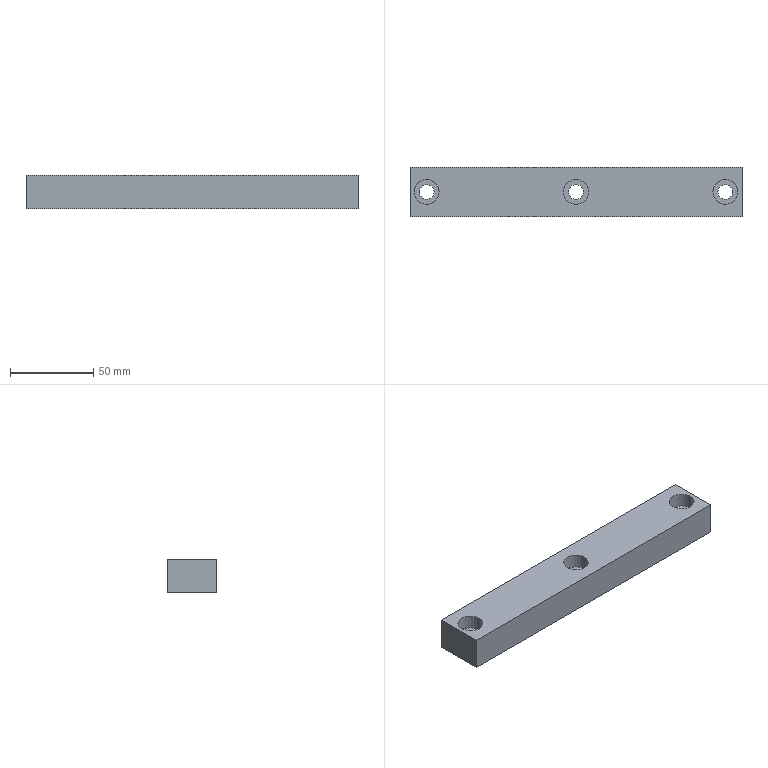Part | SolidWorks | features Extrusion 1, HoleWzd 1 | 1 solid | 21 faces | box 200 x 30 x 20 mm | volume 113265 mm3 | cylinder 12 | plane 9 | commonest cylinder face diameters 9 x6 15 x6
STEP:
#1=CARTESIAN_POINT('',(-7.5,0.,11.4));
#2=VERTEX_POINT('',#1);
#3=CARTESIAN_POINT('',(7.5,0.,11.4));
#4=VERTEX_POINT('',#3);
#5=CARTESIAN_POINT('',(0.,0.,11.4));
#6=DIRECTION('',(0.,0.,1.));
#7=DIRECTION('',(1.,0.,0.));
#8=AXIS2_PLACEMENT_3D('',#5,#6,#7);
#9=CIRCLE('',#8,7.5);
#10=EDGE_CURVE('',#2,#4,#9,.T.);
#11=ORIENTED_EDGE('',*,*,#10,.F.);
#12=CARTESIAN_POINT('',(-7.5,0.,20.));
#13=VERTEX_POINT('',#12);
#14=CARTESIAN_POINT('',(-7.5,0.,20.));
#15=DIRECTION('',(0.,0.,1.));
#16=VECTOR('',#15,1000.);
#17=LINE('',#14,#16);
#18=EDGE_CURVE('',#2,#13,#17,.T.);
#19=ORIENTED_EDGE('',*,*,#18,.T.);
#20=CARTESIAN_POINT('',(7.5,0.,20.));
#21=VERTEX_POINT('',#20);
#22=CARTESIAN_POINT('',(0.,0.,20.));
#23=DIRECTION('',(0.,0.,1.));
#24=DIRECTION('',(1.,0.,0.));
#25=AXIS2_PLACEMENT_3D('',#22,#23,#24);
#26=CIRCLE('',#25,7.5);
#27=EDGE_CURVE('',#13,#21,#26,.T.);
#28=ORIENTED_EDGE('',*,*,#27,.T.);
#29=CARTESIAN_POINT('',(7.5,0.,20.));
#30=DIRECTION('',(0.,0.,1.));
#31=VECTOR('',#30,1000.);
#32=LINE('',#29,#31);
#33=EDGE_CURVE('',#4,#21,#32,.T.);
#34=ORIENTED_EDGE('',*,*,#33,.F.);
#35=EDGE_LOOP('',(#11,#19,#28,#34));
#36=FACE_OUTER_BOUND('',#35,.T.);
#37=CARTESIAN_POINT('',(0.,0.,20.));
#38=DIRECTION('',(0.,0.,1.));
#39=DIRECTION('',(1.,0.,0.));
#40=AXIS2_PLACEMENT_3D('',#37,#38,#39);
#41=CYLINDRICAL_SURFACE('',#40,7.5);
#42=ADVANCED_FACE('',(#36),#41,.F.);
#43=CARTESIAN_POINT('',(-4.5,0.,0.));
#44=VERTEX_POINT('',#43);
#45=CARTESIAN_POINT('',(4.5,0.,0.));
#46=VERTEX_POINT('',#45);
#47=CARTESIAN_POINT('',(0.,0.,0.));
#48=DIRECTION('',(0.,0.,1.));
#49=DIRECTION('',(1.,0.,0.));
#50=AXIS2_PLACEMENT_3D('',#47,#48,#49);
#51=CIRCLE('',#50,4.5);
#52=EDGE_CURVE('',#44,#46,#51,.T.);
#53=ORIENTED_EDGE('',*,*,#52,.F.);
#54=CARTESIAN_POINT('',(-4.5,0.,11.4));
#55=VERTEX_POINT('',#54);
#56=CARTESIAN_POINT('',(-4.5,0.,20.));
#57=DIRECTION('',(0.,0.,1.));
#58=VECTOR('',#57,1000.);
#59=LINE('',#56,#58);
#60=EDGE_CURVE('',#44,#55,#59,.T.);
#61=ORIENTED_EDGE('',*,*,#60,.T.);
#62=CARTESIAN_POINT('',(4.5,0.,11.4));
#63=VERTEX_POINT('',#62);
#64=CARTESIAN_POINT('',(0.,0.,11.4));
#65=DIRECTION('',(0.,0.,1.));
#66=DIRECTION('',(1.,0.,0.));
#67=AXIS2_PLACEMENT_3D('',#64,#65,#66);
#68=CIRCLE('',#67,4.5);
#69=EDGE_CURVE('',#55,#63,#68,.T.);
#70=ORIENTED_EDGE('',*,*,#69,.T.);
#71=CARTESIAN_POINT('',(4.5,0.,20.));
#72=DIRECTION('',(0.,0.,1.));
#73=VECTOR('',#72,1000.);
#74=LINE('',#71,#73);
#75=EDGE_CURVE('',#46,#63,#74,.T.);
#76=ORIENTED_EDGE('',*,*,#75,.F.);
#77=EDGE_LOOP('',(#53,#61,#70,#76));
#78=FACE_OUTER_BOUND('',#77,.T.);
#79=CARTESIAN_POINT('',(0.,0.,20.));
#80=DIRECTION('',(0.,0.,1.));
#81=DIRECTION('',(1.,0.,0.));
#82=AXIS2_PLACEMENT_3D('',#79,#80,#81);
#83=CYLINDRICAL_SURFACE('',#82,4.5);
#84=ADVANCED_FACE('',(#78),#83,.F.);
#85=CARTESIAN_POINT('',(82.5,0.,11.4));
#86=VERTEX_POINT('',#85);
#87=CARTESIAN_POINT('',(97.5,0.,11.4));
#88=VERTEX_POINT('',#87);
#89=CARTESIAN_POINT('',(90.,0.,11.4));
#90=DIRECTION('',(0.,0.,1.));
#91=DIRECTION('',(1.,0.,0.));
#92=AXIS2_PLACEMENT_3D('',#89,#90,#91);
#93=CIRCLE('',#92,7.5);
#94=EDGE_CURVE('',#86,#88,#93,.T.);
#95=ORIENTED_EDGE('',*,*,#94,.F.);
#96=CARTESIAN_POINT('',(82.5,0.,20.));
#97=VERTEX_POINT('',#96);
#98=CARTESIAN_POINT('',(82.5,0.,20.));
#99=DIRECTION('',(0.,0.,1.));
#100=VECTOR('',#99,1000.);
#101=LINE('',#98,#100);
#102=EDGE_CURVE('',#86,#97,#101,.T.);
#103=ORIENTED_EDGE('',*,*,#102,.T.);
#104=CARTESIAN_POINT('',(97.5,0.,20.));
#105=VERTEX_POINT('',#104);
#106=CARTESIAN_POINT('',(90.,0.,20.));
#107=DIRECTION('',(0.,0.,1.));
#108=DIRECTION('',(1.,0.,0.));
#109=AXIS2_PLACEMENT_3D('',#106,#107,#108);
#110=CIRCLE('',#109,7.5);
#111=EDGE_CURVE('',#97,#105,#110,.T.);
#112=ORIENTED_EDGE('',*,*,#111,.T.);
#113=CARTESIAN_POINT('',(97.5,0.,20.));
#114=DIRECTION('',(0.,0.,1.));
#115=VECTOR('',#114,1000.);
#116=LINE('',#113,#115);
#117=EDGE_CURVE('',#88,#105,#116,.T.);
#118=ORIENTED_EDGE('',*,*,#117,.F.);
#119=EDGE_LOOP('',(#95,#103,#112,#118));
#120=FACE_OUTER_BOUND('',#119,.T.);
#121=CARTESIAN_POINT('',(90.,0.,20.));
#122=DIRECTION('',(0.,0.,1.));
#123=DIRECTION('',(1.,0.,0.));
#124=AXIS2_PLACEMENT_3D('',#121,#122,#123);
#125=CYLINDRICAL_SURFACE('',#124,7.5);
#126=ADVANCED_FACE('',(#120),#125,.F.);
#127=CARTESIAN_POINT('',(85.5,0.,0.));
#128=VERTEX_POINT('',#127);
#129=CARTESIAN_POINT('',(94.5,0.,0.));
#130=VERTEX_POINT('',#129);
#131=CARTESIAN_POINT('',(90.,0.,0.));
#132=DIRECTION('',(0.,0.,1.));
#133=DIRECTION('',(1.,0.,0.));
#134=AXIS2_PLACEMENT_3D('',#131,#132,#133);
#135=CIRCLE('',#134,4.5);
#136=EDGE_CURVE('',#128,#130,#135,.T.);
#137=ORIENTED_EDGE('',*,*,#136,.F.);
#138=CARTESIAN_POINT('',(85.5,0.,11.4));
#139=VERTEX_POINT('',#138);
#140=CARTESIAN_POINT('',(85.5,0.,20.));
#141=DIRECTION('',(0.,0.,1.));
#142=VECTOR('',#141,1000.);
#143=LINE('',#140,#142);
#144=EDGE_CURVE('',#128,#139,#143,.T.);
#145=ORIENTED_EDGE('',*,*,#144,.T.);
#146=CARTESIAN_POINT('',(94.5,0.,11.4));
#147=VERTEX_POINT('',#146);
#148=CARTESIAN_POINT('',(90.,0.,11.4));
#149=DIRECTION('',(0.,0.,1.));
#150=DIRECTION('',(1.,0.,0.));
#151=AXIS2_PLACEMENT_3D('',#148,#149,#150);
#152=CIRCLE('',#151,4.5);
#153=EDGE_CURVE('',#139,#147,#152,.T.);
#154=ORIENTED_EDGE('',*,*,#153,.T.);
#155=CARTESIAN_POINT('',(94.5,0.,20.));
#156=DIRECTION('',(0.,0.,1.));
#157=VECTOR('',#156,1000.);
#158=LINE('',#155,#157);
#159=EDGE_CURVE('',#130,#147,#158,.T.);
#160=ORIENTED_EDGE('',*,*,#159,.F.);
#161=EDGE_LOOP('',(#137,#145,#154,#160));
#162=FACE_OUTER_BOUND('',#161,.T.);
#163=CARTESIAN_POINT('',(90.,0.,20.));
#164=DIRECTION('',(0.,0.,1.));
#165=DIRECTION('',(1.,0.,0.));
#166=AXIS2_PLACEMENT_3D('',#163,#164,#165);
#167=CYLINDRICAL_SURFACE('',#166,4.5);
#168=ADVANCED_FACE('',(#162),#167,.F.);
#169=CARTESIAN_POINT('',(-97.5,0.,11.4));
#170=VERTEX_POINT('',#169);
#171=CARTESIAN_POINT('',(-82.5,0.,11.4));
#172=VERTEX_POINT('',#171);
#173=CARTESIAN_POINT('',(-90.,0.,11.4));
#174=DIRECTION('',(0.,0.,1.));
#175=DIRECTION('',(1.,0.,0.));
#176=AXIS2_PLACEMENT_3D('',#173,#174,#175);
#177=CIRCLE('',#176,7.5);
#178=EDGE_CURVE('',#170,#172,#177,.T.);
#179=ORIENTED_EDGE('',*,*,#178,.F.);
#180=CARTESIAN_POINT('',(-97.5,0.,20.));
#181=VERTEX_POINT('',#180);
#182=CARTESIAN_POINT('',(-97.5,0.,20.));
#183=DIRECTION('',(0.,0.,1.));
#184=VECTOR('',#183,1000.);
#185=LINE('',#182,#184);
#186=EDGE_CURVE('',#170,#181,#185,.T.);
#187=ORIENTED_EDGE('',*,*,#186,.T.);
#188=CARTESIAN_POINT('',(-82.5,0.,20.));
#189=VERTEX_POINT('',#188);
#190=CARTESIAN_POINT('',(-90.,0.,20.));
#191=DIRECTION('',(0.,0.,1.));
#192=DIRECTION('',(1.,0.,0.));
#193=AXIS2_PLACEMENT_3D('',#190,#191,#192);
#194=CIRCLE('',#193,7.5);
#195=EDGE_CURVE('',#181,#189,#194,.T.);
#196=ORIENTED_EDGE('',*,*,#195,.T.);
#197=CARTESIAN_POINT('',(-82.5,0.,20.));
#198=DIRECTION('',(0.,0.,1.));
#199=VECTOR('',#198,1000.);
#200=LINE('',#197,#199);
#201=EDGE_CURVE('',#172,#189,#200,.T.);
#202=ORIENTED_EDGE('',*,*,#201,.F.);
#203=EDGE_LOOP('',(#179,#187,#196,#202));
#204=FACE_OUTER_BOUND('',#203,.T.);
#205=CARTESIAN_POINT('',(-90.,0.,20.));
#206=DIRECTION('',(0.,0.,1.));
#207=DIRECTION('',(1.,0.,0.));
#208=AXIS2_PLACEMENT_3D('',#205,#206,#207);
#209=CYLINDRICAL_SURFACE('',#208,7.5);
#210=ADVANCED_FACE('',(#204),#209,.F.);
#211=CARTESIAN_POINT('',(-94.5,0.,0.));
#212=VERTEX_POINT('',#211);
#213=CARTESIAN_POINT('',(-85.5,0.,0.));
#214=VERTEX_POINT('',#213);
#215=CARTESIAN_POINT('',(-90.,0.,0.));
#216=DIRECTION('',(0.,0.,1.));
#217=DIRECTION('',(1.,0.,0.));
#218=AXIS2_PLACEMENT_3D('',#215,#216,#217);
#219=CIRCLE('',#218,4.5);
#220=EDGE_CURVE('',#212,#214,#219,.T.);
#221=ORIENTED_EDGE('',*,*,#220,.F.);
#222=CARTESIAN_POINT('',(-94.5,0.,11.4));
#223=VERTEX_POINT('',#222);
#224=CARTESIAN_POINT('',(-94.5,0.,20.));
#225=DIRECTION('',(0.,0.,1.));
#226=VECTOR('',#225,1000.);
#227=LINE('',#224,#226);
#228=EDGE_CURVE('',#212,#223,#227,.T.);
#229=ORIENTED_EDGE('',*,*,#228,.T.);
#230=CARTESIAN_POINT('',(-85.5,0.,11.4));
#231=VERTEX_POINT('',#230);
#232=CARTESIAN_POINT('',(-90.,0.,11.4));
#233=DIRECTION('',(0.,0.,1.));
#234=DIRECTION('',(1.,0.,0.));
#235=AXIS2_PLACEMENT_3D('',#232,#233,#234);
#236=CIRCLE('',#235,4.5);
#237=EDGE_CURVE('',#223,#231,#236,.T.);
#238=ORIENTED_EDGE('',*,*,#237,.T.);
#239=CARTESIAN_POINT('',(-85.5,0.,20.));
#240=DIRECTION('',(0.,0.,1.));
#241=VECTOR('',#240,1000.);
#242=LINE('',#239,#241);
#243=EDGE_CURVE('',#214,#231,#242,.T.);
#244=ORIENTED_EDGE('',*,*,#243,.F.);
#245=EDGE_LOOP('',(#221,#229,#238,#244));
#246=FACE_OUTER_BOUND('',#245,.T.);
#247=CARTESIAN_POINT('',(-90.,0.,20.));
#248=DIRECTION('',(0.,0.,1.));
#249=DIRECTION('',(1.,0.,0.));
#250=AXIS2_PLACEMENT_3D('',#247,#248,#249);
#251=CYLINDRICAL_SURFACE('',#250,4.5);
#252=ADVANCED_FACE('',(#246),#251,.F.);
#253=CARTESIAN_POINT('',(100.,-15.,0.));
#254=VERTEX_POINT('',#253);
#255=CARTESIAN_POINT('',(100.,15.,0.));
#256=VERTEX_POINT('',#255);
#257=CARTESIAN_POINT('',(100.,-15.,0.));
#258=DIRECTION('',(0.,1.,0.));
#259=VECTOR('',#258,1000.);
#260=LINE('',#257,#259);
#261=EDGE_CURVE('',#254,#256,#260,.T.);
#262=ORIENTED_EDGE('',*,*,#261,.T.);
#263=CARTESIAN_POINT('',(100.,15.,20.));
#264=VERTEX_POINT('',#263);
#265=CARTESIAN_POINT('',(100.,15.,20.));
#266=DIRECTION('',(0.,0.,-1.));
#267=VECTOR('',#266,1000.);
#268=LINE('',#265,#267);
#269=EDGE_CURVE('',#264,#256,#268,.T.);
#270=ORIENTED_EDGE('',*,*,#269,.F.);
#271=CARTESIAN_POINT('',(100.,-15.,20.));
#272=VERTEX_POINT('',#271);
#273=CARTESIAN_POINT('',(100.,-15.,20.));
#274=DIRECTION('',(0.,1.,0.));
#275=VECTOR('',#274,1000.);
#276=LINE('',#273,#275);
#277=EDGE_CURVE('',#272,#264,#276,.T.);
#278=ORIENTED_EDGE('',*,*,#277,.F.);
#279=CARTESIAN_POINT('',(100.,-15.,20.));
#280=DIRECTION('',(0.,0.,-1.));
#281=VECTOR('',#280,1000.);
#282=LINE('',#279,#281);
#283=EDGE_CURVE('',#272,#254,#282,.T.);
#284=ORIENTED_EDGE('',*,*,#283,.T.);
#285=EDGE_LOOP('',(#262,#270,#278,#284));
#286=FACE_OUTER_BOUND('',#285,.T.);
#287=CARTESIAN_POINT('',(100.,-15.,20.));
#288=DIRECTION('',(-1.,0.,0.));
#289=DIRECTION('',(0.,0.,1.));
#290=AXIS2_PLACEMENT_3D('',#287,#288,#289);
#291=PLANE('',#290);
#292=ADVANCED_FACE('',(#286),#291,.F.);
#293=CARTESIAN_POINT('',(-100.,15.,0.));
#294=VERTEX_POINT('',#293);
#295=CARTESIAN_POINT('',(-100.,15.,0.));
#296=DIRECTION('',(-1.,0.,0.));
#297=VECTOR('',#296,1000.);
#298=LINE('',#295,#297);
#299=EDGE_CURVE('',#256,#294,#298,.T.);
#300=ORIENTED_EDGE('',*,*,#299,.T.);
#301=CARTESIAN_POINT('',(-100.,15.,20.));
#302=VERTEX_POINT('',#301);
#303=CARTESIAN_POINT('',(-100.,15.,20.));
#304=DIRECTION('',(0.,0.,-1.));
#305=VECTOR('',#304,1000.);
#306=LINE('',#303,#305);
#307=EDGE_CURVE('',#302,#294,#306,.T.);
#308=ORIENTED_EDGE('',*,*,#307,.F.);
#309=CARTESIAN_POINT('',(-100.,15.,20.));
#310=DIRECTION('',(-1.,0.,0.));
#311=VECTOR('',#310,1000.);
#312=LINE('',#309,#311);
#313=EDGE_CURVE('',#264,#302,#312,.T.);
#314=ORIENTED_EDGE('',*,*,#313,.F.);
#315=ORIENTED_EDGE('',*,*,#269,.T.);
#316=EDGE_LOOP('',(#300,#308,#314,#315));
#317=FACE_OUTER_BOUND('',#316,.T.);
#318=CARTESIAN_POINT('',(-100.,15.,20.));
#319=DIRECTION('',(0.,-1.,0.));
#320=DIRECTION('',(0.,0.,-1.));
#321=AXIS2_PLACEMENT_3D('',#318,#319,#320);
#322=PLANE('',#321);
#323=ADVANCED_FACE('',(#317),#322,.F.);
#324=CARTESIAN_POINT('',(-100.,-15.,0.));
#325=VERTEX_POINT('',#324);
#326=CARTESIAN_POINT('',(-100.,-15.,0.));
#327=DIRECTION('',(0.,-1.,0.));
#328=VECTOR('',#327,1000.);
#329=LINE('',#326,#328);
#330=EDGE_CURVE('',#294,#325,#329,.T.);
#331=ORIENTED_EDGE('',*,*,#330,.T.);
#332=CARTESIAN_POINT('',(-100.,-15.,20.));
#333=VERTEX_POINT('',#332);
#334=CARTESIAN_POINT('',(-100.,-15.,20.));
#335=DIRECTION('',(0.,0.,-1.));
#336=VECTOR('',#335,1000.);
#337=LINE('',#334,#336);
#338=EDGE_CURVE('',#333,#325,#337,.T.);
#339=ORIENTED_EDGE('',*,*,#338,.F.);
#340=CARTESIAN_POINT('',(-100.,-15.,20.));
#341=DIRECTION('',(0.,-1.,0.));
#342=VECTOR('',#341,1000.);
#343=LINE('',#340,#342);
#344=EDGE_CURVE('',#302,#333,#343,.T.);
#345=ORIENTED_EDGE('',*,*,#344,.F.);
#346=ORIENTED_EDGE('',*,*,#307,.T.);
#347=EDGE_LOOP('',(#331,#339,#345,#346));
#348=FACE_OUTER_BOUND('',#347,.T.);
#349=CARTESIAN_POINT('',(-100.,-15.,20.));
#350=DIRECTION('',(1.,0.,0.));
#351=DIRECTION('',(0.,0.,-1.));
#352=AXIS2_PLACEMENT_3D('',#349,#350,#351);
#353=PLANE('',#352);
#354=ADVANCED_FACE('',(#348),#353,.F.);
#355=CARTESIAN_POINT('',(-100.,-15.,0.));
#356=DIRECTION('',(1.,0.,0.));
#357=VECTOR('',#356,1000.);
#358=LINE('',#355,#357);
#359=EDGE_CURVE('',#325,#254,#358,.T.);
#360=ORIENTED_EDGE('',*,*,#359,.T.);
#361=ORIENTED_EDGE('',*,*,#283,.F.);
#362=CARTESIAN_POINT('',(-100.,-15.,20.));
#363=DIRECTION('',(1.,0.,0.));
#364=VECTOR('',#363,1000.);
#365=LINE('',#362,#364);
#366=EDGE_CURVE('',#333,#272,#365,.T.);
#367=ORIENTED_EDGE('',*,*,#366,.F.);
#368=ORIENTED_EDGE('',*,*,#338,.T.);
#369=EDGE_LOOP('',(#360,#361,#367,#368));
#370=FACE_OUTER_BOUND('',#369,.T.);
#371=CARTESIAN_POINT('',(-100.,-15.,20.));
#372=DIRECTION('',(0.,1.,0.));
#373=DIRECTION('',(0.,0.,1.));
#374=AXIS2_PLACEMENT_3D('',#371,#372,#373);
#375=PLANE('',#374);
#376=ADVANCED_FACE('',(#370),#375,.F.);
#377=CARTESIAN_POINT('',(0.,0.,20.));
#378=DIRECTION('',(0.,0.,1.));
#379=DIRECTION('',(1.,0.,0.));
#380=AXIS2_PLACEMENT_3D('',#377,#378,#379);
#381=CIRCLE('',#380,7.5);
#382=EDGE_CURVE('',#21,#13,#381,.T.);
#383=ORIENTED_EDGE('',*,*,#382,.F.);
#384=ORIENTED_EDGE('',*,*,#27,.F.);
#385=EDGE_LOOP('',(#383,#384));
#386=FACE_BOUND('',#385,.T.);
#387=CARTESIAN_POINT('',(90.,0.,20.));
#388=DIRECTION('',(0.,0.,1.));
#389=DIRECTION('',(1.,0.,0.));
#390=AXIS2_PLACEMENT_3D('',#387,#388,#389);
#391=CIRCLE('',#390,7.5);
#392=EDGE_CURVE('',#105,#97,#391,.T.);
#393=ORIENTED_EDGE('',*,*,#392,.F.);
#394=ORIENTED_EDGE('',*,*,#111,.F.);
#395=EDGE_LOOP('',(#393,#394));
#396=FACE_BOUND('',#395,.T.);
#397=CARTESIAN_POINT('',(-90.,0.,20.));
#398=DIRECTION('',(0.,0.,1.));
#399=DIRECTION('',(1.,0.,0.));
#400=AXIS2_PLACEMENT_3D('',#397,#398,#399);
#401=CIRCLE('',#400,7.5);
#402=EDGE_CURVE('',#189,#181,#401,.T.);
#403=ORIENTED_EDGE('',*,*,#402,.F.);
#404=ORIENTED_EDGE('',*,*,#195,.F.);
#405=EDGE_LOOP('',(#403,#404));
#406=FACE_BOUND('',#405,.T.);
#407=ORIENTED_EDGE('',*,*,#277,.T.);
#408=ORIENTED_EDGE('',*,*,#313,.T.);
#409=ORIENTED_EDGE('',*,*,#344,.T.);
#410=ORIENTED_EDGE('',*,*,#366,.T.);
#411=EDGE_LOOP('',(#407,#408,#409,#410));
#412=FACE_OUTER_BOUND('',#411,.T.);
#413=CARTESIAN_POINT('',(0.,0.,20.));
#414=DIRECTION('',(0.,0.,-1.));
#415=DIRECTION('',(-1.,0.,0.));
#416=AXIS2_PLACEMENT_3D('',#413,#414,#415);
#417=PLANE('',#416);
#418=ADVANCED_FACE('',(#386,#396,#406,#412),#417,.F.);
#419=CARTESIAN_POINT('',(0.,0.,0.));
#420=DIRECTION('',(0.,0.,1.));
#421=DIRECTION('',(1.,0.,0.));
#422=AXIS2_PLACEMENT_3D('',#419,#420,#421);
#423=CIRCLE('',#422,4.5);
#424=EDGE_CURVE('',#46,#44,#423,.T.);
#425=ORIENTED_EDGE('',*,*,#424,.T.);
#426=ORIENTED_EDGE('',*,*,#52,.T.);
#427=EDGE_LOOP('',(#425,#426));
#428=FACE_BOUND('',#427,.T.);
#429=CARTESIAN_POINT('',(90.,0.,0.));
#430=DIRECTION('',(0.,0.,1.));
#431=DIRECTION('',(1.,0.,0.));
#432=AXIS2_PLACEMENT_3D('',#429,#430,#431);
#433=CIRCLE('',#432,4.5);
#434=EDGE_CURVE('',#130,#128,#433,.T.);
#435=ORIENTED_EDGE('',*,*,#434,.T.);
#436=ORIENTED_EDGE('',*,*,#136,.T.);
#437=EDGE_LOOP('',(#435,#436));
#438=FACE_BOUND('',#437,.T.);
#439=CARTESIAN_POINT('',(-90.,0.,0.));
#440=DIRECTION('',(0.,0.,1.));
#441=DIRECTION('',(1.,0.,0.));
#442=AXIS2_PLACEMENT_3D('',#439,#440,#441);
#443=CIRCLE('',#442,4.5);
#444=EDGE_CURVE('',#214,#212,#443,.T.);
#445=ORIENTED_EDGE('',*,*,#444,.T.);
#446=ORIENTED_EDGE('',*,*,#220,.T.);
#447=EDGE_LOOP('',(#445,#446));
#448=FACE_BOUND('',#447,.T.);
#449=ORIENTED_EDGE('',*,*,#261,.F.);
#450=ORIENTED_EDGE('',*,*,#359,.F.);
#451=ORIENTED_EDGE('',*,*,#330,.F.);
#452=ORIENTED_EDGE('',*,*,#299,.F.);
#453=EDGE_LOOP('',(#449,#450,#451,#452));
#454=FACE_OUTER_BOUND('',#453,.T.);
#455=CARTESIAN_POINT('',(0.,0.,0.));
#456=DIRECTION('',(0.,0.,-1.));
#457=DIRECTION('',(-1.,0.,0.));
#458=AXIS2_PLACEMENT_3D('',#455,#456,#457);
#459=PLANE('',#458);
#460=ADVANCED_FACE('',(#428,#438,#448,#454),#459,.T.);
#461=ORIENTED_EDGE('',*,*,#228,.F.);
#462=ORIENTED_EDGE('',*,*,#444,.F.);
#463=ORIENTED_EDGE('',*,*,#243,.T.);
#464=CARTESIAN_POINT('',(-90.,0.,11.4));
#465=DIRECTION('',(0.,0.,1.));
#466=DIRECTION('',(1.,0.,0.));
#467=AXIS2_PLACEMENT_3D('',#464,#465,#466);
#468=CIRCLE('',#467,4.5);
#469=EDGE_CURVE('',#231,#223,#468,.T.);
#470=ORIENTED_EDGE('',*,*,#469,.T.);
#471=EDGE_LOOP('',(#461,#462,#463,#470));
#472=FACE_OUTER_BOUND('',#471,.T.);
#473=CARTESIAN_POINT('',(-90.,0.,20.));
#474=DIRECTION('',(0.,0.,1.));
#475=DIRECTION('',(1.,0.,0.));
#476=AXIS2_PLACEMENT_3D('',#473,#474,#475);
#477=CYLINDRICAL_SURFACE('',#476,4.5);
#478=ADVANCED_FACE('',(#472),#477,.F.);
#479=ORIENTED_EDGE('',*,*,#469,.F.);
#480=ORIENTED_EDGE('',*,*,#237,.F.);
#481=EDGE_LOOP('',(#479,#480));
#482=FACE_BOUND('',#481,.T.);
#483=CARTESIAN_POINT('',(-90.,0.,11.4));
#484=DIRECTION('',(0.,0.,1.));
#485=DIRECTION('',(1.,0.,0.));
#486=AXIS2_PLACEMENT_3D('',#483,#484,#485);
#487=CIRCLE('',#486,7.5);
#488=EDGE_CURVE('',#172,#170,#487,.T.);
#489=ORIENTED_EDGE('',*,*,#488,.T.);
#490=ORIENTED_EDGE('',*,*,#178,.T.);
#491=EDGE_LOOP('',(#489,#490));
#492=FACE_OUTER_BOUND('',#491,.T.);
#493=CARTESIAN_POINT('',(-85.5,0.,11.4));
#494=DIRECTION('',(0.,0.,-1.));
#495=DIRECTION('',(-1.,0.,0.));
#496=AXIS2_PLACEMENT_3D('',#493,#494,#495);
#497=PLANE('',#496);
#498=ADVANCED_FACE('',(#482,#492),#497,.F.);
#499=ORIENTED_EDGE('',*,*,#186,.F.);
#500=ORIENTED_EDGE('',*,*,#488,.F.);
#501=ORIENTED_EDGE('',*,*,#201,.T.);
#502=ORIENTED_EDGE('',*,*,#402,.T.);
#503=EDGE_LOOP('',(#499,#500,#501,#502));
#504=FACE_OUTER_BOUND('',#503,.T.);
#505=CARTESIAN_POINT('',(-90.,0.,20.));
#506=DIRECTION('',(0.,0.,1.));
#507=DIRECTION('',(1.,0.,0.));
#508=AXIS2_PLACEMENT_3D('',#505,#506,#507);
#509=CYLINDRICAL_SURFACE('',#508,7.5);
#510=ADVANCED_FACE('',(#504),#509,.F.);
#511=ORIENTED_EDGE('',*,*,#144,.F.);
#512=ORIENTED_EDGE('',*,*,#434,.F.);
#513=ORIENTED_EDGE('',*,*,#159,.T.);
#514=CARTESIAN_POINT('',(90.,0.,11.4));
#515=DIRECTION('',(0.,0.,1.));
#516=DIRECTION('',(1.,0.,0.));
#517=AXIS2_PLACEMENT_3D('',#514,#515,#516);
#518=CIRCLE('',#517,4.5);
#519=EDGE_CURVE('',#147,#139,#518,.T.);
#520=ORIENTED_EDGE('',*,*,#519,.T.);
#521=EDGE_LOOP('',(#511,#512,#513,#520));
#522=FACE_OUTER_BOUND('',#521,.T.);
#523=CARTESIAN_POINT('',(90.,0.,20.));
#524=DIRECTION('',(0.,0.,1.));
#525=DIRECTION('',(1.,0.,0.));
#526=AXIS2_PLACEMENT_3D('',#523,#524,#525);
#527=CYLINDRICAL_SURFACE('',#526,4.5);
#528=ADVANCED_FACE('',(#522),#527,.F.);
#529=ORIENTED_EDGE('',*,*,#519,.F.);
#530=ORIENTED_EDGE('',*,*,#153,.F.);
#531=EDGE_LOOP('',(#529,#530));
#532=FACE_BOUND('',#531,.T.);
#533=CARTESIAN_POINT('',(90.,0.,11.4));
#534=DIRECTION('',(0.,0.,1.));
#535=DIRECTION('',(1.,0.,0.));
#536=AXIS2_PLACEMENT_3D('',#533,#534,#535);
#537=CIRCLE('',#536,7.5);
#538=EDGE_CURVE('',#88,#86,#537,.T.);
#539=ORIENTED_EDGE('',*,*,#538,.T.);
#540=ORIENTED_EDGE('',*,*,#94,.T.);
#541=EDGE_LOOP('',(#539,#540));
#542=FACE_OUTER_BOUND('',#541,.T.);
#543=CARTESIAN_POINT('',(94.5,0.,11.4));
#544=DIRECTION('',(0.,0.,-1.));
#545=DIRECTION('',(-1.,0.,0.));
#546=AXIS2_PLACEMENT_3D('',#543,#544,#545);
#547=PLANE('',#546);
#548=ADVANCED_FACE('',(#532,#542),#547,.F.);
#549=ORIENTED_EDGE('',*,*,#102,.F.);
#550=ORIENTED_EDGE('',*,*,#538,.F.);
#551=ORIENTED_EDGE('',*,*,#117,.T.);
#552=ORIENTED_EDGE('',*,*,#392,.T.);
#553=EDGE_LOOP('',(#549,#550,#551,#552));
#554=FACE_OUTER_BOUND('',#553,.T.);
#555=CARTESIAN_POINT('',(90.,0.,20.));
#556=DIRECTION('',(0.,0.,1.));
#557=DIRECTION('',(1.,0.,0.));
#558=AXIS2_PLACEMENT_3D('',#555,#556,#557);
#559=CYLINDRICAL_SURFACE('',#558,7.5);
#560=ADVANCED_FACE('',(#554),#559,.F.);
#561=ORIENTED_EDGE('',*,*,#60,.F.);
#562=ORIENTED_EDGE('',*,*,#424,.F.);
#563=ORIENTED_EDGE('',*,*,#75,.T.);
#564=CARTESIAN_POINT('',(0.,0.,11.4));
#565=DIRECTION('',(0.,0.,1.));
#566=DIRECTION('',(1.,0.,0.));
#567=AXIS2_PLACEMENT_3D('',#564,#565,#566);
#568=CIRCLE('',#567,4.5);
#569=EDGE_CURVE('',#63,#55,#568,.T.);
#570=ORIENTED_EDGE('',*,*,#569,.T.);
#571=EDGE_LOOP('',(#561,#562,#563,#570));
#572=FACE_OUTER_BOUND('',#571,.T.);
#573=CARTESIAN_POINT('',(0.,0.,20.));
#574=DIRECTION('',(0.,0.,1.));
#575=DIRECTION('',(1.,0.,0.));
#576=AXIS2_PLACEMENT_3D('',#573,#574,#575);
#577=CYLINDRICAL_SURFACE('',#576,4.5);
#578=ADVANCED_FACE('',(#572),#577,.F.);
#579=ORIENTED_EDGE('',*,*,#569,.F.);
#580=ORIENTED_EDGE('',*,*,#69,.F.);
#581=EDGE_LOOP('',(#579,#580));
#582=FACE_BOUND('',#581,.T.);
#583=CARTESIAN_POINT('',(0.,0.,11.4));
#584=DIRECTION('',(0.,0.,1.));
#585=DIRECTION('',(1.,0.,0.));
#586=AXIS2_PLACEMENT_3D('',#583,#584,#585);
#587=CIRCLE('',#586,7.5);
#588=EDGE_CURVE('',#4,#2,#587,.T.);
#589=ORIENTED_EDGE('',*,*,#588,.T.);
#590=ORIENTED_EDGE('',*,*,#10,.T.);
#591=EDGE_LOOP('',(#589,#590));
#592=FACE_OUTER_BOUND('',#591,.T.);
#593=CARTESIAN_POINT('',(4.5,0.,11.4));
#594=DIRECTION('',(0.,0.,-1.));
#595=DIRECTION('',(-1.,0.,0.));
#596=AXIS2_PLACEMENT_3D('',#593,#594,#595);
#597=PLANE('',#596);
#598=ADVANCED_FACE('',(#582,#592),#597,.F.);
#599=ORIENTED_EDGE('',*,*,#18,.F.);
#600=ORIENTED_EDGE('',*,*,#588,.F.);
#601=ORIENTED_EDGE('',*,*,#33,.T.);
#602=ORIENTED_EDGE('',*,*,#382,.T.);
#603=EDGE_LOOP('',(#599,#600,#601,#602));
#604=FACE_OUTER_BOUND('',#603,.T.);
#605=CARTESIAN_POINT('',(0.,0.,20.));
#606=DIRECTION('',(0.,0.,1.));
#607=DIRECTION('',(1.,0.,0.));
#608=AXIS2_PLACEMENT_3D('',#605,#606,#607);
#609=CYLINDRICAL_SURFACE('',#608,7.5);
#610=ADVANCED_FACE('',(#604),#609,.F.);
#611=CLOSED_SHELL('',(#42,#84,#126,#168,#210,#252,#292,#323,#354,#376,#418,#460,#478,#498,#510,#528,#548,#560,#578,#598,#610));
#612=MANIFOLD_SOLID_BREP('',#611);
#613=CARTESIAN_POINT('',(0.,0.,0.));
#614=DIRECTION('',(0.,0.,1.));
#615=DIRECTION('',(1.,0.,0.));
#616=AXIS2_PLACEMENT_3D('',#613,#614,#615);
#617=(LENGTH_UNIT()NAMED_UNIT(*)SI_UNIT(.MILLI.,.METRE.));
#618=UNCERTAINTY_MEASURE_WITH_UNIT(LENGTH_MEASURE(0.00001),#617,'','');
#619=(NAMED_UNIT(*)PLANE_ANGLE_UNIT()SI_UNIT($,.RADIAN.));
#620=(NAMED_UNIT(*)SI_UNIT($,.STERADIAN.)SOLID_ANGLE_UNIT());
#621=(GEOMETRIC_REPRESENTATION_CONTEXT(3)GLOBAL_UNCERTAINTY_ASSIGNED_CONTEXT((#618))GLOBAL_UNIT_ASSIGNED_CONTEXT((#617,#619,#620))REPRESENTATION_CONTEXT('',''));
#622=ADVANCED_BREP_SHAPE_REPRESENTATION('',(#612,#616),#621);